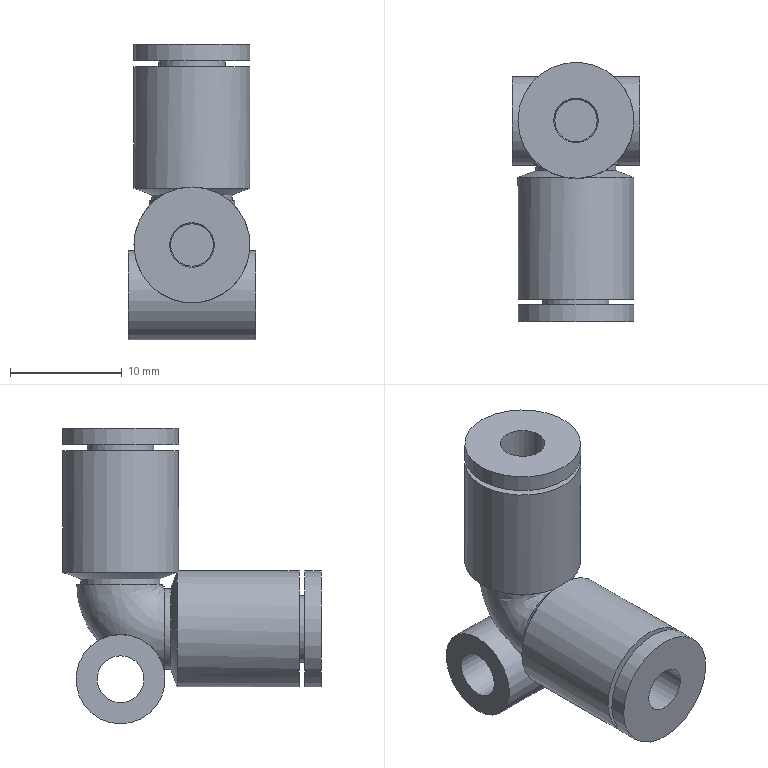Part | NX | 1 solid | 29 faces | box 11.4 x 23.2 x 26.5 mm | volume 2503 mm3 | cylinder 12 | plane 12 | cone 4 | spline 1 | commonest cylinder face diameters 10.4 x4 4 x2 6 x2 7.2 x2 4.2 x1 8 x1